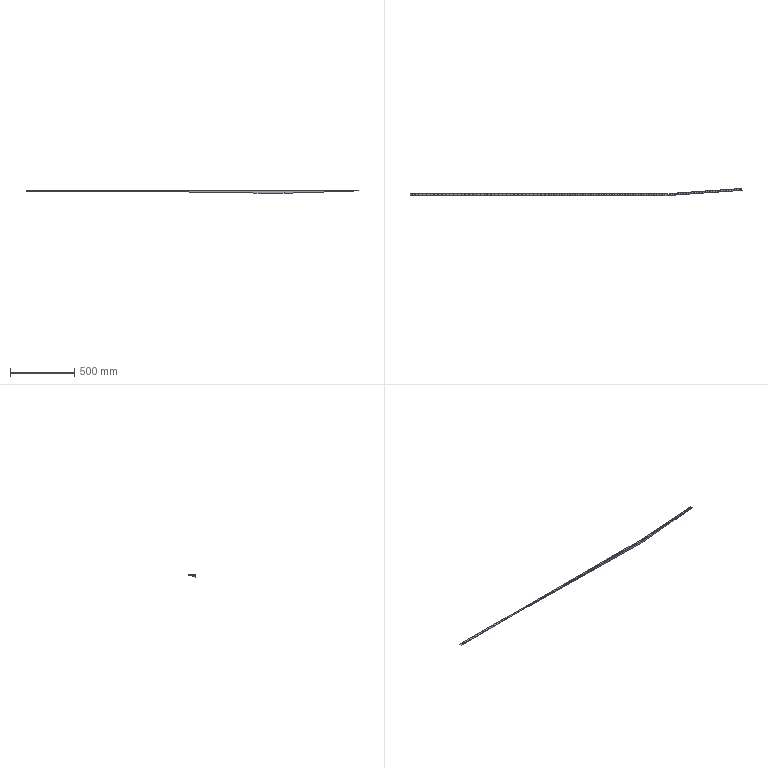Part | SolidWorks | features BaseBody 1 | 1 solid | 236 faces | box 2579 x 55.207 x 21.862 mm | volume 171026 mm3 | cylinder 220 | plane 16 | commonest cylinder face diameters 3.2 x220